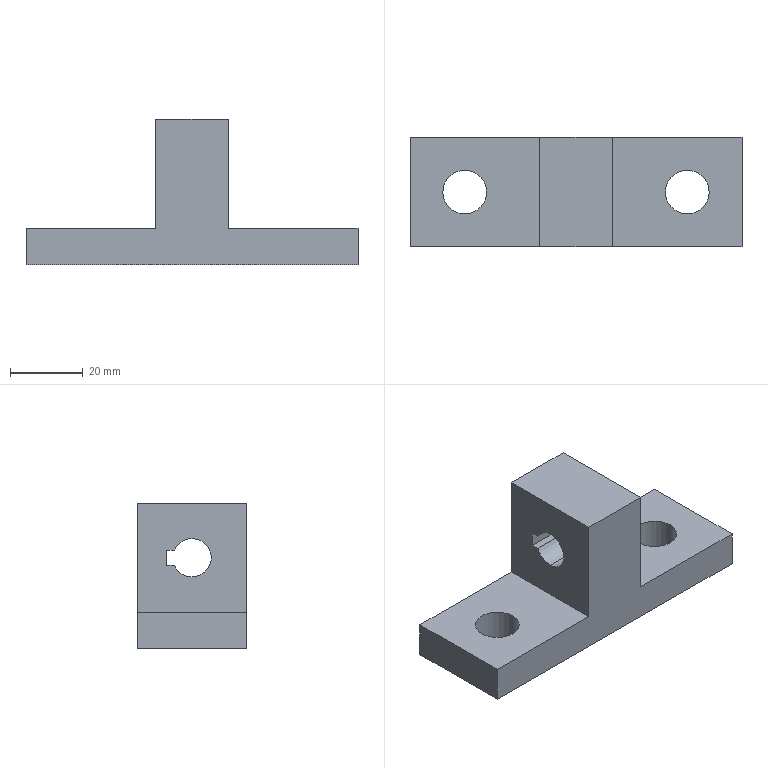Part | SolidWorks | features ICE 3, Extrusion 1 | 1 solid | 20 faces | box 91 x 30 x 40 mm | volume 41147 mm3 | plane 13 | cylinder 7 | commonest cylinder face diameters 12 x4 10.5 x3
STEP:
#1=CARTESIAN_POINT('',(-24.5,0.,0.));
#2=VERTEX_POINT('',#1);
#3=CARTESIAN_POINT('',(-36.5,0.,0.));
#4=VERTEX_POINT('',#3);
#5=CARTESIAN_POINT('',(-30.5,0.,0.));
#6=DIRECTION('',(0.,0.,-1.));
#7=DIRECTION('',(-1.,0.,0.));
#8=AXIS2_PLACEMENT_3D('',#5,#6,#7);
#9=CIRCLE('',#8,6.);
#10=EDGE_CURVE('',#2,#4,#9,.T.);
#11=ORIENTED_EDGE('',*,*,#10,.T.);
#12=CARTESIAN_POINT('',(-36.5,0.,10.));
#13=VERTEX_POINT('',#12);
#14=CARTESIAN_POINT('',(-36.5,0.,-20.));
#15=DIRECTION('',(0.,0.,1.));
#16=VECTOR('',#15,1000.);
#17=LINE('',#14,#16);
#18=EDGE_CURVE('',#4,#13,#17,.T.);
#19=ORIENTED_EDGE('',*,*,#18,.T.);
#20=CARTESIAN_POINT('',(-24.5,0.,10.));
#21=VERTEX_POINT('',#20);
#22=CARTESIAN_POINT('',(-30.5,0.,10.));
#23=DIRECTION('',(0.,0.,1.));
#24=DIRECTION('',(1.,0.,0.));
#25=AXIS2_PLACEMENT_3D('',#22,#23,#24);
#26=CIRCLE('',#25,6.);
#27=EDGE_CURVE('',#13,#21,#26,.T.);
#28=ORIENTED_EDGE('',*,*,#27,.T.);
#29=CARTESIAN_POINT('',(-24.5,0.,-20.));
#30=DIRECTION('',(0.,0.,1.));
#31=VECTOR('',#30,1000.);
#32=LINE('',#29,#31);
#33=EDGE_CURVE('',#2,#21,#32,.T.);
#34=ORIENTED_EDGE('',*,*,#33,.F.);
#35=EDGE_LOOP('',(#11,#19,#28,#34));
#36=FACE_OUTER_BOUND('',#35,.T.);
#37=CARTESIAN_POINT('',(-30.5,0.,-20.));
#38=DIRECTION('',(0.,0.,1.));
#39=DIRECTION('',(1.,0.,0.));
#40=AXIS2_PLACEMENT_3D('',#37,#38,#39);
#41=CYLINDRICAL_SURFACE('',#40,6.);
#42=ADVANCED_FACE('',(#36),#41,.F.);
#43=CARTESIAN_POINT('',(36.5,0.,0.));
#44=VERTEX_POINT('',#43);
#45=CARTESIAN_POINT('',(24.5,0.,0.));
#46=VERTEX_POINT('',#45);
#47=CARTESIAN_POINT('',(30.5,0.,0.));
#48=DIRECTION('',(0.,0.,-1.));
#49=DIRECTION('',(-1.,0.,0.));
#50=AXIS2_PLACEMENT_3D('',#47,#48,#49);
#51=CIRCLE('',#50,6.);
#52=EDGE_CURVE('',#44,#46,#51,.T.);
#53=ORIENTED_EDGE('',*,*,#52,.T.);
#54=CARTESIAN_POINT('',(24.5,0.,10.));
#55=VERTEX_POINT('',#54);
#56=CARTESIAN_POINT('',(24.5,0.,-20.));
#57=DIRECTION('',(0.,0.,1.));
#58=VECTOR('',#57,1000.);
#59=LINE('',#56,#58);
#60=EDGE_CURVE('',#46,#55,#59,.T.);
#61=ORIENTED_EDGE('',*,*,#60,.T.);
#62=CARTESIAN_POINT('',(36.5,0.,10.));
#63=VERTEX_POINT('',#62);
#64=CARTESIAN_POINT('',(30.5,0.,10.));
#65=DIRECTION('',(0.,0.,1.));
#66=DIRECTION('',(-1.,0.,0.));
#67=AXIS2_PLACEMENT_3D('',#64,#65,#66);
#68=CIRCLE('',#67,6.);
#69=EDGE_CURVE('',#55,#63,#68,.T.);
#70=ORIENTED_EDGE('',*,*,#69,.T.);
#71=CARTESIAN_POINT('',(36.5,0.,-20.));
#72=DIRECTION('',(0.,0.,1.));
#73=VECTOR('',#72,1000.);
#74=LINE('',#71,#73);
#75=EDGE_CURVE('',#44,#63,#74,.T.);
#76=ORIENTED_EDGE('',*,*,#75,.F.);
#77=EDGE_LOOP('',(#53,#61,#70,#76));
#78=FACE_OUTER_BOUND('',#77,.T.);
#79=CARTESIAN_POINT('',(30.5,0.,-20.));
#80=DIRECTION('',(0.,0.,1.));
#81=DIRECTION('',(1.,0.,0.));
#82=AXIS2_PLACEMENT_3D('',#79,#80,#81);
#83=CYLINDRICAL_SURFACE('',#82,6.);
#84=ADVANCED_FACE('',(#78),#83,.F.);
#85=CARTESIAN_POINT('',(10.,0.,19.75));
#86=VERTEX_POINT('',#85);
#87=CARTESIAN_POINT('',(10.,0.,30.25));
#88=VERTEX_POINT('',#87);
#89=CARTESIAN_POINT('',(10.,0.,25.));
#90=DIRECTION('',(-1.,0.,0.));
#91=DIRECTION('',(0.,0.,1.));
#92=AXIS2_PLACEMENT_3D('',#89,#90,#91);
#93=CIRCLE('',#92,5.25);
#94=EDGE_CURVE('',#86,#88,#93,.T.);
#95=ORIENTED_EDGE('',*,*,#94,.F.);
#96=CARTESIAN_POINT('',(-10.,0.,19.75));
#97=VERTEX_POINT('',#96);
#98=CARTESIAN_POINT('',(20.,0.,19.75));
#99=DIRECTION('',(-1.,0.,0.));
#100=VECTOR('',#99,1000.);
#101=LINE('',#98,#100);
#102=EDGE_CURVE('',#86,#97,#101,.T.);
#103=ORIENTED_EDGE('',*,*,#102,.T.);
#104=CARTESIAN_POINT('',(-10.,0.,30.25));
#105=VERTEX_POINT('',#104);
#106=CARTESIAN_POINT('',(-10.,0.,25.));
#107=DIRECTION('',(-1.,0.,0.));
#108=DIRECTION('',(0.,0.,1.));
#109=AXIS2_PLACEMENT_3D('',#106,#107,#108);
#110=CIRCLE('',#109,5.25);
#111=EDGE_CURVE('',#97,#105,#110,.T.);
#112=ORIENTED_EDGE('',*,*,#111,.T.);
#113=CARTESIAN_POINT('',(20.,0.,30.25));
#114=DIRECTION('',(-1.,0.,0.));
#115=VECTOR('',#114,1000.);
#116=LINE('',#113,#115);
#117=EDGE_CURVE('',#88,#105,#116,.T.);
#118=ORIENTED_EDGE('',*,*,#117,.F.);
#119=EDGE_LOOP('',(#95,#103,#112,#118));
#120=FACE_OUTER_BOUND('',#119,.T.);
#121=CARTESIAN_POINT('',(20.,0.,25.));
#122=DIRECTION('',(-1.,0.,0.));
#123=DIRECTION('',(0.,0.,1.));
#124=AXIS2_PLACEMENT_3D('',#121,#122,#123);
#125=CYLINDRICAL_SURFACE('',#124,5.25);
#126=ADVANCED_FACE('',(#120),#125,.F.);
#127=CARTESIAN_POINT('',(10.,4.812,27.1));
#128=VERTEX_POINT('',#127);
#129=CARTESIAN_POINT('',(10.,0.,25.));
#130=DIRECTION('',(-1.,0.,0.));
#131=DIRECTION('',(0.,0.,1.));
#132=AXIS2_PLACEMENT_3D('',#129,#130,#131);
#133=CIRCLE('',#132,5.25);
#134=EDGE_CURVE('',#88,#128,#133,.T.);
#135=ORIENTED_EDGE('',*,*,#134,.F.);
#136=ORIENTED_EDGE('',*,*,#117,.T.);
#137=CARTESIAN_POINT('',(-10.,4.812,27.1));
#138=VERTEX_POINT('',#137);
#139=CARTESIAN_POINT('',(-10.,0.,25.));
#140=DIRECTION('',(-1.,0.,0.));
#141=DIRECTION('',(0.,0.,1.));
#142=AXIS2_PLACEMENT_3D('',#139,#140,#141);
#143=CIRCLE('',#142,5.25);
#144=EDGE_CURVE('',#105,#138,#143,.T.);
#145=ORIENTED_EDGE('',*,*,#144,.T.);
#146=CARTESIAN_POINT('',(20.,4.812,27.1));
#147=DIRECTION('',(-1.,0.,0.));
#148=VECTOR('',#147,1000.);
#149=LINE('',#146,#148);
#150=EDGE_CURVE('',#128,#138,#149,.T.);
#151=ORIENTED_EDGE('',*,*,#150,.F.);
#152=EDGE_LOOP('',(#135,#136,#145,#151));
#153=FACE_OUTER_BOUND('',#152,.T.);
#154=CARTESIAN_POINT('',(20.,0.,25.));
#155=DIRECTION('',(-1.,0.,0.));
#156=DIRECTION('',(0.,0.,1.));
#157=AXIS2_PLACEMENT_3D('',#154,#155,#156);
#158=CYLINDRICAL_SURFACE('',#157,5.25);
#159=ADVANCED_FACE('',(#153),#158,.F.);
#160=CARTESIAN_POINT('',(30.5,0.,10.));
#161=DIRECTION('',(0.,0.,1.));
#162=DIRECTION('',(-1.,0.,0.));
#163=AXIS2_PLACEMENT_3D('',#160,#161,#162);
#164=CIRCLE('',#163,6.);
#165=EDGE_CURVE('',#63,#55,#164,.T.);
#166=ORIENTED_EDGE('',*,*,#165,.F.);
#167=ORIENTED_EDGE('',*,*,#69,.F.);
#168=EDGE_LOOP('',(#166,#167));
#169=FACE_BOUND('',#168,.T.);
#170=CARTESIAN_POINT('',(10.,-15.,10.));
#171=VERTEX_POINT('',#170);
#172=CARTESIAN_POINT('',(10.,15.,10.));
#173=VERTEX_POINT('',#172);
#174=CARTESIAN_POINT('',(10.,-15.,10.));
#175=DIRECTION('',(0.,1.,0.));
#176=VECTOR('',#175,1000.);
#177=LINE('',#174,#176);
#178=EDGE_CURVE('',#171,#173,#177,.T.);
#179=ORIENTED_EDGE('',*,*,#178,.F.);
#180=CARTESIAN_POINT('',(45.5,-15.,10.));
#181=VERTEX_POINT('',#180);
#182=CARTESIAN_POINT('',(-45.5,-15.,10.));
#183=DIRECTION('',(1.,0.,0.));
#184=VECTOR('',#183,1000.);
#185=LINE('',#182,#184);
#186=EDGE_CURVE('',#171,#181,#185,.T.);
#187=ORIENTED_EDGE('',*,*,#186,.T.);
#188=CARTESIAN_POINT('',(45.5,15.,10.));
#189=VERTEX_POINT('',#188);
#190=CARTESIAN_POINT('',(45.5,-15.,10.));
#191=DIRECTION('',(0.,1.,0.));
#192=VECTOR('',#191,1000.);
#193=LINE('',#190,#192);
#194=EDGE_CURVE('',#181,#189,#193,.T.);
#195=ORIENTED_EDGE('',*,*,#194,.T.);
#196=CARTESIAN_POINT('',(-45.5,15.,10.));
#197=DIRECTION('',(-1.,0.,0.));
#198=VECTOR('',#197,1000.);
#199=LINE('',#196,#198);
#200=EDGE_CURVE('',#189,#173,#199,.T.);
#201=ORIENTED_EDGE('',*,*,#200,.T.);
#202=EDGE_LOOP('',(#179,#187,#195,#201));
#203=FACE_OUTER_BOUND('',#202,.T.);
#204=CARTESIAN_POINT('',(0.,0.,10.));
#205=DIRECTION('',(0.,0.,-1.));
#206=DIRECTION('',(-1.,0.,0.));
#207=AXIS2_PLACEMENT_3D('',#204,#205,#206);
#208=PLANE('',#207);
#209=ADVANCED_FACE('',(#169,#203),#208,.F.);
#210=CARTESIAN_POINT('',(-30.5,0.,10.));
#211=DIRECTION('',(0.,0.,1.));
#212=DIRECTION('',(1.,0.,0.));
#213=AXIS2_PLACEMENT_3D('',#210,#211,#212);
#214=CIRCLE('',#213,6.);
#215=EDGE_CURVE('',#21,#13,#214,.T.);
#216=ORIENTED_EDGE('',*,*,#215,.F.);
#217=ORIENTED_EDGE('',*,*,#27,.F.);
#218=EDGE_LOOP('',(#216,#217));
#219=FACE_BOUND('',#218,.T.);
#220=CARTESIAN_POINT('',(-10.,15.,10.));
#221=VERTEX_POINT('',#220);
#222=CARTESIAN_POINT('',(-10.,-15.,10.));
#223=VERTEX_POINT('',#222);
#224=CARTESIAN_POINT('',(-10.,-15.,10.));
#225=DIRECTION('',(0.,-1.,0.));
#226=VECTOR('',#225,1000.);
#227=LINE('',#224,#226);
#228=EDGE_CURVE('',#221,#223,#227,.T.);
#229=ORIENTED_EDGE('',*,*,#228,.F.);
#230=CARTESIAN_POINT('',(-45.5,15.,10.));
#231=VERTEX_POINT('',#230);
#232=CARTESIAN_POINT('',(-45.5,15.,10.));
#233=DIRECTION('',(-1.,0.,0.));
#234=VECTOR('',#233,1000.);
#235=LINE('',#232,#234);
#236=EDGE_CURVE('',#221,#231,#235,.T.);
#237=ORIENTED_EDGE('',*,*,#236,.T.);
#238=CARTESIAN_POINT('',(-45.5,-15.,10.));
#239=VERTEX_POINT('',#238);
#240=CARTESIAN_POINT('',(-45.5,-15.,10.));
#241=DIRECTION('',(0.,-1.,0.));
#242=VECTOR('',#241,1000.);
#243=LINE('',#240,#242);
#244=EDGE_CURVE('',#231,#239,#243,.T.);
#245=ORIENTED_EDGE('',*,*,#244,.T.);
#246=CARTESIAN_POINT('',(-45.5,-15.,10.));
#247=DIRECTION('',(1.,0.,0.));
#248=VECTOR('',#247,1000.);
#249=LINE('',#246,#248);
#250=EDGE_CURVE('',#239,#223,#249,.T.);
#251=ORIENTED_EDGE('',*,*,#250,.T.);
#252=EDGE_LOOP('',(#229,#237,#245,#251));
#253=FACE_OUTER_BOUND('',#252,.T.);
#254=CARTESIAN_POINT('',(0.,0.,10.));
#255=DIRECTION('',(0.,0.,-1.));
#256=DIRECTION('',(-1.,0.,0.));
#257=AXIS2_PLACEMENT_3D('',#254,#255,#256);
#258=PLANE('',#257);
#259=ADVANCED_FACE('',(#219,#253),#258,.F.);
#260=CARTESIAN_POINT('',(45.5,-15.,0.));
#261=VERTEX_POINT('',#260);
#262=CARTESIAN_POINT('',(45.5,15.,0.));
#263=VERTEX_POINT('',#262);
#264=CARTESIAN_POINT('',(45.5,-15.,0.));
#265=DIRECTION('',(0.,1.,0.));
#266=VECTOR('',#265,1000.);
#267=LINE('',#264,#266);
#268=EDGE_CURVE('',#261,#263,#267,.T.);
#269=ORIENTED_EDGE('',*,*,#268,.T.);
#270=CARTESIAN_POINT('',(45.5,15.,10.));
#271=DIRECTION('',(0.,0.,-1.));
#272=VECTOR('',#271,1000.);
#273=LINE('',#270,#272);
#274=EDGE_CURVE('',#189,#263,#273,.T.);
#275=ORIENTED_EDGE('',*,*,#274,.F.);
#276=ORIENTED_EDGE('',*,*,#194,.F.);
#277=CARTESIAN_POINT('',(45.5,-15.,10.));
#278=DIRECTION('',(0.,0.,-1.));
#279=VECTOR('',#278,1000.);
#280=LINE('',#277,#279);
#281=EDGE_CURVE('',#181,#261,#280,.T.);
#282=ORIENTED_EDGE('',*,*,#281,.T.);
#283=EDGE_LOOP('',(#269,#275,#276,#282));
#284=FACE_OUTER_BOUND('',#283,.T.);
#285=CARTESIAN_POINT('',(45.5,-15.,10.));
#286=DIRECTION('',(-1.,0.,0.));
#287=DIRECTION('',(0.,0.,1.));
#288=AXIS2_PLACEMENT_3D('',#285,#286,#287);
#289=PLANE('',#288);
#290=ADVANCED_FACE('',(#284),#289,.F.);
#291=CARTESIAN_POINT('',(-45.5,15.,0.));
#292=VERTEX_POINT('',#291);
#293=CARTESIAN_POINT('',(-45.5,15.,0.));
#294=DIRECTION('',(-1.,0.,0.));
#295=VECTOR('',#294,1000.);
#296=LINE('',#293,#295);
#297=EDGE_CURVE('',#263,#292,#296,.T.);
#298=ORIENTED_EDGE('',*,*,#297,.T.);
#299=CARTESIAN_POINT('',(-45.5,15.,10.));
#300=DIRECTION('',(0.,0.,-1.));
#301=VECTOR('',#300,1000.);
#302=LINE('',#299,#301);
#303=EDGE_CURVE('',#231,#292,#302,.T.);
#304=ORIENTED_EDGE('',*,*,#303,.F.);
#305=ORIENTED_EDGE('',*,*,#236,.F.);
#306=CARTESIAN_POINT('',(-10.,15.,40.));
#307=VERTEX_POINT('',#306);
#308=CARTESIAN_POINT('',(-10.,15.,40.));
#309=DIRECTION('',(0.,0.,-1.));
#310=VECTOR('',#309,1000.);
#311=LINE('',#308,#310);
#312=EDGE_CURVE('',#307,#221,#311,.T.);
#313=ORIENTED_EDGE('',*,*,#312,.F.);
#314=CARTESIAN_POINT('',(10.,15.,40.));
#315=VERTEX_POINT('',#314);
#316=CARTESIAN_POINT('',(-10.,15.,40.));
#317=DIRECTION('',(-1.,0.,0.));
#318=VECTOR('',#317,1000.);
#319=LINE('',#316,#318);
#320=EDGE_CURVE('',#315,#307,#319,.T.);
#321=ORIENTED_EDGE('',*,*,#320,.F.);
#322=CARTESIAN_POINT('',(10.,15.,40.));
#323=DIRECTION('',(0.,0.,-1.));
#324=VECTOR('',#323,1000.);
#325=LINE('',#322,#324);
#326=EDGE_CURVE('',#315,#173,#325,.T.);
#327=ORIENTED_EDGE('',*,*,#326,.T.);
#328=ORIENTED_EDGE('',*,*,#200,.F.);
#329=ORIENTED_EDGE('',*,*,#274,.T.);
#330=EDGE_LOOP('',(#298,#304,#305,#313,#321,#327,#328,#329));
#331=FACE_OUTER_BOUND('',#330,.T.);
#332=CARTESIAN_POINT('',(-45.5,15.,10.));
#333=DIRECTION('',(0.,-1.,0.));
#334=DIRECTION('',(0.,0.,-1.));
#335=AXIS2_PLACEMENT_3D('',#332,#333,#334);
#336=PLANE('',#335);
#337=ADVANCED_FACE('',(#331),#336,.F.);
#338=CARTESIAN_POINT('',(-45.5,-15.,0.));
#339=VERTEX_POINT('',#338);
#340=CARTESIAN_POINT('',(-45.5,-15.,0.));
#341=DIRECTION('',(0.,-1.,0.));
#342=VECTOR('',#341,1000.);
#343=LINE('',#340,#342);
#344=EDGE_CURVE('',#292,#339,#343,.T.);
#345=ORIENTED_EDGE('',*,*,#344,.T.);
#346=CARTESIAN_POINT('',(-45.5,-15.,10.));
#347=DIRECTION('',(0.,0.,-1.));
#348=VECTOR('',#347,1000.);
#349=LINE('',#346,#348);
#350=EDGE_CURVE('',#239,#339,#349,.T.);
#351=ORIENTED_EDGE('',*,*,#350,.F.);
#352=ORIENTED_EDGE('',*,*,#244,.F.);
#353=ORIENTED_EDGE('',*,*,#303,.T.);
#354=EDGE_LOOP('',(#345,#351,#352,#353));
#355=FACE_OUTER_BOUND('',#354,.T.);
#356=CARTESIAN_POINT('',(-45.5,-15.,10.));
#357=DIRECTION('',(1.,0.,0.));
#358=DIRECTION('',(0.,0.,-1.));
#359=AXIS2_PLACEMENT_3D('',#356,#357,#358);
#360=PLANE('',#359);
#361=ADVANCED_FACE('',(#355),#360,.F.);
#362=CARTESIAN_POINT('',(-45.5,-15.,0.));
#363=DIRECTION('',(1.,0.,0.));
#364=VECTOR('',#363,1000.);
#365=LINE('',#362,#364);
#366=EDGE_CURVE('',#339,#261,#365,.T.);
#367=ORIENTED_EDGE('',*,*,#366,.T.);
#368=ORIENTED_EDGE('',*,*,#281,.F.);
#369=ORIENTED_EDGE('',*,*,#186,.F.);
#370=CARTESIAN_POINT('',(10.,-15.,40.));
#371=VERTEX_POINT('',#370);
#372=CARTESIAN_POINT('',(10.,-15.,40.));
#373=DIRECTION('',(0.,0.,-1.));
#374=VECTOR('',#373,1000.);
#375=LINE('',#372,#374);
#376=EDGE_CURVE('',#371,#171,#375,.T.);
#377=ORIENTED_EDGE('',*,*,#376,.F.);
#378=CARTESIAN_POINT('',(-10.,-15.,40.));
#379=VERTEX_POINT('',#378);
#380=CARTESIAN_POINT('',(-10.,-15.,40.));
#381=DIRECTION('',(1.,0.,0.));
#382=VECTOR('',#381,1000.);
#383=LINE('',#380,#382);
#384=EDGE_CURVE('',#379,#371,#383,.T.);
#385=ORIENTED_EDGE('',*,*,#384,.F.);
#386=CARTESIAN_POINT('',(-10.,-15.,40.));
#387=DIRECTION('',(0.,0.,-1.));
#388=VECTOR('',#387,1000.);
#389=LINE('',#386,#388);
#390=EDGE_CURVE('',#379,#223,#389,.T.);
#391=ORIENTED_EDGE('',*,*,#390,.T.);
#392=ORIENTED_EDGE('',*,*,#250,.F.);
#393=ORIENTED_EDGE('',*,*,#350,.T.);
#394=EDGE_LOOP('',(#367,#368,#369,#377,#385,#391,#392,#393));
#395=FACE_OUTER_BOUND('',#394,.T.);
#396=CARTESIAN_POINT('',(-45.5,-15.,10.));
#397=DIRECTION('',(0.,1.,0.));
#398=DIRECTION('',(0.,0.,1.));
#399=AXIS2_PLACEMENT_3D('',#396,#397,#398);
#400=PLANE('',#399);
#401=ADVANCED_FACE('',(#395),#400,.F.);
#402=ORIENTED_EDGE('',*,*,#10,.F.);
#403=CARTESIAN_POINT('',(-30.5,0.,0.));
#404=DIRECTION('',(0.,0.,-1.));
#405=DIRECTION('',(-1.,0.,0.));
#406=AXIS2_PLACEMENT_3D('',#403,#404,#405);
#407=CIRCLE('',#406,6.);
#408=EDGE_CURVE('',#4,#2,#407,.T.);
#409=ORIENTED_EDGE('',*,*,#408,.F.);
#410=EDGE_LOOP('',(#402,#409));
#411=FACE_BOUND('',#410,.T.);
#412=ORIENTED_EDGE('',*,*,#52,.F.);
#413=CARTESIAN_POINT('',(30.5,0.,0.));
#414=DIRECTION('',(0.,0.,-1.));
#415=DIRECTION('',(-1.,0.,0.));
#416=AXIS2_PLACEMENT_3D('',#413,#414,#415);
#417=CIRCLE('',#416,6.);
#418=EDGE_CURVE('',#46,#44,#417,.T.);
#419=ORIENTED_EDGE('',*,*,#418,.F.);
#420=EDGE_LOOP('',(#412,#419));
#421=FACE_BOUND('',#420,.T.);
#422=ORIENTED_EDGE('',*,*,#268,.F.);
#423=ORIENTED_EDGE('',*,*,#366,.F.);
#424=ORIENTED_EDGE('',*,*,#344,.F.);
#425=ORIENTED_EDGE('',*,*,#297,.F.);
#426=EDGE_LOOP('',(#422,#423,#424,#425));
#427=FACE_OUTER_BOUND('',#426,.T.);
#428=CARTESIAN_POINT('',(0.,0.,0.));
#429=DIRECTION('',(0.,0.,-1.));
#430=DIRECTION('',(-1.,0.,0.));
#431=AXIS2_PLACEMENT_3D('',#428,#429,#430);
#432=PLANE('',#431);
#433=ADVANCED_FACE('',(#411,#421,#427),#432,.T.);
#434=CARTESIAN_POINT('',(10.,4.812,22.9));
#435=VERTEX_POINT('',#434);
#436=CARTESIAN_POINT('',(10.,0.,25.));
#437=DIRECTION('',(-1.,0.,0.));
#438=DIRECTION('',(0.,0.,1.));
#439=AXIS2_PLACEMENT_3D('',#436,#437,#438);
#440=CIRCLE('',#439,5.25);
#441=EDGE_CURVE('',#435,#86,#440,.T.);
#442=ORIENTED_EDGE('',*,*,#441,.T.);
#443=ORIENTED_EDGE('',*,*,#94,.T.);
#444=ORIENTED_EDGE('',*,*,#134,.T.);
#445=CARTESIAN_POINT('',(10.,7.,27.1));
#446=VERTEX_POINT('',#445);
#447=CARTESIAN_POINT('',(10.,-15.,27.1));
#448=DIRECTION('',(0.,1.,0.));
#449=VECTOR('',#448,1000.);
#450=LINE('',#447,#449);
#451=EDGE_CURVE('',#128,#446,#450,.T.);
#452=ORIENTED_EDGE('',*,*,#451,.T.);
#453=CARTESIAN_POINT('',(10.,7.,22.9));
#454=VERTEX_POINT('',#453);
#455=CARTESIAN_POINT('',(10.,7.,40.));
#456=DIRECTION('',(0.,0.,-1.));
#457=VECTOR('',#456,1000.);
#458=LINE('',#455,#457);
#459=EDGE_CURVE('',#446,#454,#458,.T.);
#460=ORIENTED_EDGE('',*,*,#459,.T.);
#461=CARTESIAN_POINT('',(10.,-15.,22.9));
#462=DIRECTION('',(0.,-1.,0.));
#463=VECTOR('',#462,1000.);
#464=LINE('',#461,#463);
#465=EDGE_CURVE('',#454,#435,#464,.T.);
#466=ORIENTED_EDGE('',*,*,#465,.T.);
#467=EDGE_LOOP('',(#442,#443,#444,#452,#460,#466));
#468=FACE_BOUND('',#467,.T.);
#469=ORIENTED_EDGE('',*,*,#178,.T.);
#470=ORIENTED_EDGE('',*,*,#326,.F.);
#471=CARTESIAN_POINT('',(10.,-15.,40.));
#472=DIRECTION('',(0.,1.,0.));
#473=VECTOR('',#472,1000.);
#474=LINE('',#471,#473);
#475=EDGE_CURVE('',#371,#315,#474,.T.);
#476=ORIENTED_EDGE('',*,*,#475,.F.);
#477=ORIENTED_EDGE('',*,*,#376,.T.);
#478=EDGE_LOOP('',(#469,#470,#476,#477));
#479=FACE_OUTER_BOUND('',#478,.T.);
#480=CARTESIAN_POINT('',(10.,-15.,40.));
#481=DIRECTION('',(-1.,0.,0.));
#482=DIRECTION('',(0.,0.,1.));
#483=AXIS2_PLACEMENT_3D('',#480,#481,#482);
#484=PLANE('',#483);
#485=ADVANCED_FACE('',(#468,#479),#484,.F.);
#486=CARTESIAN_POINT('',(-10.,7.,27.1));
#487=VERTEX_POINT('',#486);
#488=CARTESIAN_POINT('',(-10.,7.,22.9));
#489=VERTEX_POINT('',#488);
#490=CARTESIAN_POINT('',(-10.,7.,27.1));
#491=DIRECTION('',(0.,0.,-1.));
#492=VECTOR('',#491,1000.);
#493=LINE('',#490,#492);
#494=EDGE_CURVE('',#487,#489,#493,.T.);
#495=ORIENTED_EDGE('',*,*,#494,.F.);
#496=CARTESIAN_POINT('',(-10.,7.,27.1));
#497=DIRECTION('',(0.,1.,0.));
#498=VECTOR('',#497,1000.);
#499=LINE('',#496,#498);
#500=EDGE_CURVE('',#138,#487,#499,.T.);
#501=ORIENTED_EDGE('',*,*,#500,.F.);
#502=ORIENTED_EDGE('',*,*,#144,.F.);
#503=ORIENTED_EDGE('',*,*,#111,.F.);
#504=CARTESIAN_POINT('',(-10.,4.812,22.9));
#505=VERTEX_POINT('',#504);
#506=CARTESIAN_POINT('',(-10.,0.,25.));
#507=DIRECTION('',(-1.,0.,0.));
#508=DIRECTION('',(0.,0.,1.));
#509=AXIS2_PLACEMENT_3D('',#506,#507,#508);
#510=CIRCLE('',#509,5.25);
#511=EDGE_CURVE('',#505,#97,#510,.T.);
#512=ORIENTED_EDGE('',*,*,#511,.F.);
#513=CARTESIAN_POINT('',(-10.,7.,22.9));
#514=DIRECTION('',(0.,-1.,0.));
#515=VECTOR('',#514,1000.);
#516=LINE('',#513,#515);
#517=EDGE_CURVE('',#489,#505,#516,.T.);
#518=ORIENTED_EDGE('',*,*,#517,.F.);
#519=EDGE_LOOP('',(#495,#501,#502,#503,#512,#518));
#520=FACE_BOUND('',#519,.T.);
#521=ORIENTED_EDGE('',*,*,#228,.T.);
#522=ORIENTED_EDGE('',*,*,#390,.F.);
#523=CARTESIAN_POINT('',(-10.,-15.,40.));
#524=DIRECTION('',(0.,-1.,0.));
#525=VECTOR('',#524,1000.);
#526=LINE('',#523,#525);
#527=EDGE_CURVE('',#307,#379,#526,.T.);
#528=ORIENTED_EDGE('',*,*,#527,.F.);
#529=ORIENTED_EDGE('',*,*,#312,.T.);
#530=EDGE_LOOP('',(#521,#522,#528,#529));
#531=FACE_OUTER_BOUND('',#530,.T.);
#532=CARTESIAN_POINT('',(-10.,-15.,40.));
#533=DIRECTION('',(1.,0.,0.));
#534=DIRECTION('',(0.,0.,-1.));
#535=AXIS2_PLACEMENT_3D('',#532,#533,#534);
#536=PLANE('',#535);
#537=ADVANCED_FACE('',(#520,#531),#536,.F.);
#538=ORIENTED_EDGE('',*,*,#475,.T.);
#539=ORIENTED_EDGE('',*,*,#320,.T.);
#540=ORIENTED_EDGE('',*,*,#527,.T.);
#541=ORIENTED_EDGE('',*,*,#384,.T.);
#542=EDGE_LOOP('',(#538,#539,#540,#541));
#543=FACE_OUTER_BOUND('',#542,.T.);
#544=CARTESIAN_POINT('',(0.,0.,40.));
#545=DIRECTION('',(0.,0.,-1.));
#546=DIRECTION('',(-1.,0.,0.));
#547=AXIS2_PLACEMENT_3D('',#544,#545,#546);
#548=PLANE('',#547);
#549=ADVANCED_FACE('',(#543),#548,.F.);
#550=ORIENTED_EDGE('',*,*,#150,.T.);
#551=ORIENTED_EDGE('',*,*,#500,.T.);
#552=CARTESIAN_POINT('',(20.,7.,27.1));
#553=DIRECTION('',(-1.,0.,0.));
#554=VECTOR('',#553,1000.);
#555=LINE('',#552,#554);
#556=EDGE_CURVE('',#446,#487,#555,.T.);
#557=ORIENTED_EDGE('',*,*,#556,.F.);
#558=ORIENTED_EDGE('',*,*,#451,.F.);
#559=EDGE_LOOP('',(#550,#551,#557,#558));
#560=FACE_OUTER_BOUND('',#559,.T.);
#561=CARTESIAN_POINT('',(20.,7.,27.1));
#562=DIRECTION('',(0.,0.,1.));
#563=DIRECTION('',(1.,0.,0.));
#564=AXIS2_PLACEMENT_3D('',#561,#562,#563);
#565=PLANE('',#564);
#566=ADVANCED_FACE('',(#560),#565,.F.);
#567=ORIENTED_EDGE('',*,*,#102,.F.);
#568=ORIENTED_EDGE('',*,*,#441,.F.);
#569=CARTESIAN_POINT('',(20.,4.812,22.9));
#570=DIRECTION('',(-1.,0.,0.));
#571=VECTOR('',#570,1000.);
#572=LINE('',#569,#571);
#573=EDGE_CURVE('',#435,#505,#572,.T.);
#574=ORIENTED_EDGE('',*,*,#573,.T.);
#575=ORIENTED_EDGE('',*,*,#511,.T.);
#576=EDGE_LOOP('',(#567,#568,#574,#575));
#577=FACE_OUTER_BOUND('',#576,.T.);
#578=CARTESIAN_POINT('',(20.,0.,25.));
#579=DIRECTION('',(-1.,0.,0.));
#580=DIRECTION('',(0.,0.,1.));
#581=AXIS2_PLACEMENT_3D('',#578,#579,#580);
#582=CYLINDRICAL_SURFACE('',#581,5.25);
#583=ADVANCED_FACE('',(#577),#582,.F.);
#584=CARTESIAN_POINT('',(20.,7.,22.9));
#585=DIRECTION('',(-1.,0.,0.));
#586=VECTOR('',#585,1000.);
#587=LINE('',#584,#586);
#588=EDGE_CURVE('',#454,#489,#587,.T.);
#589=ORIENTED_EDGE('',*,*,#588,.T.);
#590=ORIENTED_EDGE('',*,*,#517,.T.);
#591=ORIENTED_EDGE('',*,*,#573,.F.);
#592=ORIENTED_EDGE('',*,*,#465,.F.);
#593=EDGE_LOOP('',(#589,#590,#591,#592));
#594=FACE_OUTER_BOUND('',#593,.T.);
#595=CARTESIAN_POINT('',(20.,7.,22.9));
#596=DIRECTION('',(0.,0.,-1.));
#597=DIRECTION('',(0.,1.,0.));
#598=AXIS2_PLACEMENT_3D('',#595,#596,#597);
#599=PLANE('',#598);
#600=ADVANCED_FACE('',(#594),#599,.F.);
#601=ORIENTED_EDGE('',*,*,#556,.T.);
#602=ORIENTED_EDGE('',*,*,#494,.T.);
#603=ORIENTED_EDGE('',*,*,#588,.F.);
#604=ORIENTED_EDGE('',*,*,#459,.F.);
#605=EDGE_LOOP('',(#601,#602,#603,#604));
#606=FACE_OUTER_BOUND('',#605,.T.);
#607=CARTESIAN_POINT('',(20.,7.,27.1));
#608=DIRECTION('',(0.,1.,0.));
#609=DIRECTION('',(0.,0.,1.));
#610=AXIS2_PLACEMENT_3D('',#607,#608,#609);
#611=PLANE('',#610);
#612=ADVANCED_FACE('',(#606),#611,.F.);
#613=ORIENTED_EDGE('',*,*,#60,.F.);
#614=ORIENTED_EDGE('',*,*,#418,.T.);
#615=ORIENTED_EDGE('',*,*,#75,.T.);
#616=ORIENTED_EDGE('',*,*,#165,.T.);
#617=EDGE_LOOP('',(#613,#614,#615,#616));
#618=FACE_OUTER_BOUND('',#617,.T.);
#619=CARTESIAN_POINT('',(30.5,0.,-20.));
#620=DIRECTION('',(0.,0.,1.));
#621=DIRECTION('',(1.,0.,0.));
#622=AXIS2_PLACEMENT_3D('',#619,#620,#621);
#623=CYLINDRICAL_SURFACE('',#622,6.);
#624=ADVANCED_FACE('',(#618),#623,.F.);
#625=ORIENTED_EDGE('',*,*,#18,.F.);
#626=ORIENTED_EDGE('',*,*,#408,.T.);
#627=ORIENTED_EDGE('',*,*,#33,.T.);
#628=ORIENTED_EDGE('',*,*,#215,.T.);
#629=EDGE_LOOP('',(#625,#626,#627,#628));
#630=FACE_OUTER_BOUND('',#629,.T.);
#631=CARTESIAN_POINT('',(-30.5,0.,-20.));
#632=DIRECTION('',(0.,0.,1.));
#633=DIRECTION('',(1.,0.,0.));
#634=AXIS2_PLACEMENT_3D('',#631,#632,#633);
#635=CYLINDRICAL_SURFACE('',#634,6.);
#636=ADVANCED_FACE('',(#630),#635,.F.);
#637=CLOSED_SHELL('',(#42,#84,#126,#159,#209,#259,#290,#337,#361,#401,#433,#485,#537,#549,#566,#583,#600,#612,#624,#636));
#638=MANIFOLD_SOLID_BREP('',#637);
#639=CARTESIAN_POINT('',(0.,0.,0.));
#640=DIRECTION('',(0.,0.,1.));
#641=DIRECTION('',(1.,0.,0.));
#642=AXIS2_PLACEMENT_3D('',#639,#640,#641);
#643=(LENGTH_UNIT()NAMED_UNIT(*)SI_UNIT(.MILLI.,.METRE.));
#644=UNCERTAINTY_MEASURE_WITH_UNIT(LENGTH_MEASURE(0.00001),#643,'','');
#645=(NAMED_UNIT(*)PLANE_ANGLE_UNIT()SI_UNIT($,.RADIAN.));
#646=(NAMED_UNIT(*)SI_UNIT($,.STERADIAN.)SOLID_ANGLE_UNIT());
#647=(GEOMETRIC_REPRESENTATION_CONTEXT(3)GLOBAL_UNCERTAINTY_ASSIGNED_CONTEXT((#644))GLOBAL_UNIT_ASSIGNED_CONTEXT((#643,#645,#646))REPRESENTATION_CONTEXT('',''));
#648=ADVANCED_BREP_SHAPE_REPRESENTATION('',(#638,#642),#647);